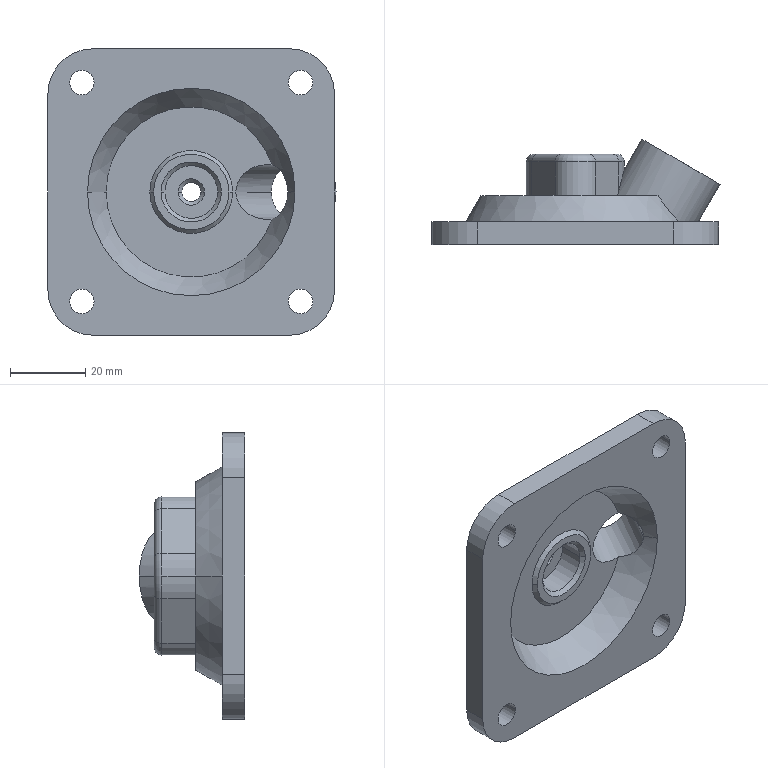Part | SolidWorks | features BaseBody 1 | 1 solid | 67 faces | box 76.392 x 28 x 76 mm | volume 42214 mm3 | cylinder 31 | plane 17 | cone 14 | torus 5 | commonest cylinder face diameters 6.5 x8 24 x6 4 x4 26 x3 5 x2 12 x2